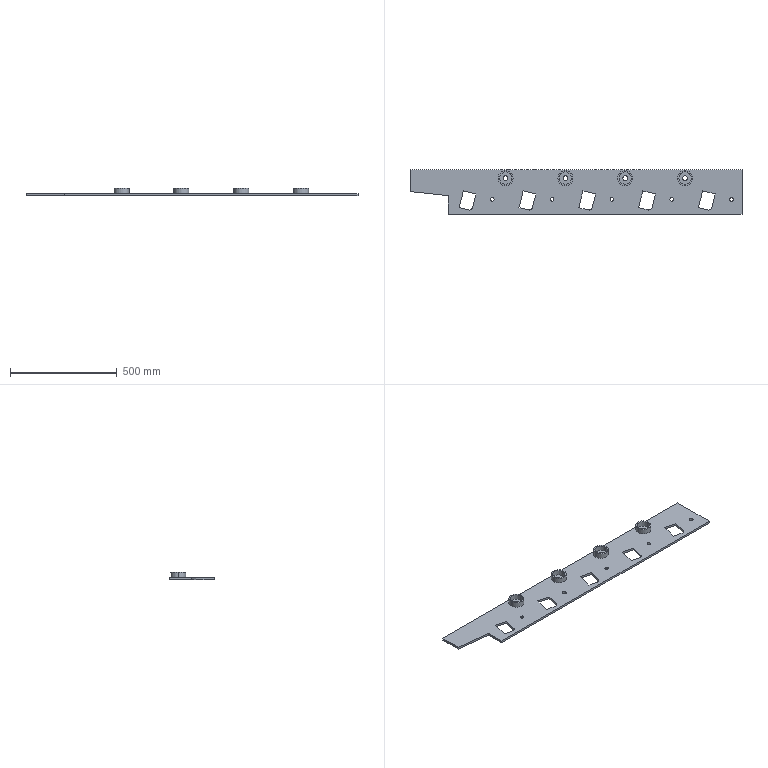Part | STEP file | Edge plate 3_Default<As machined> | 5 solids | 75 faces | box 1554 x 210 x 35 mm | volume 2937527 mm3 | cylinder 39 | plane 36 | commonest cylinder face diameters 17 x10 22 x8 58 x8 70 x8 30 x5